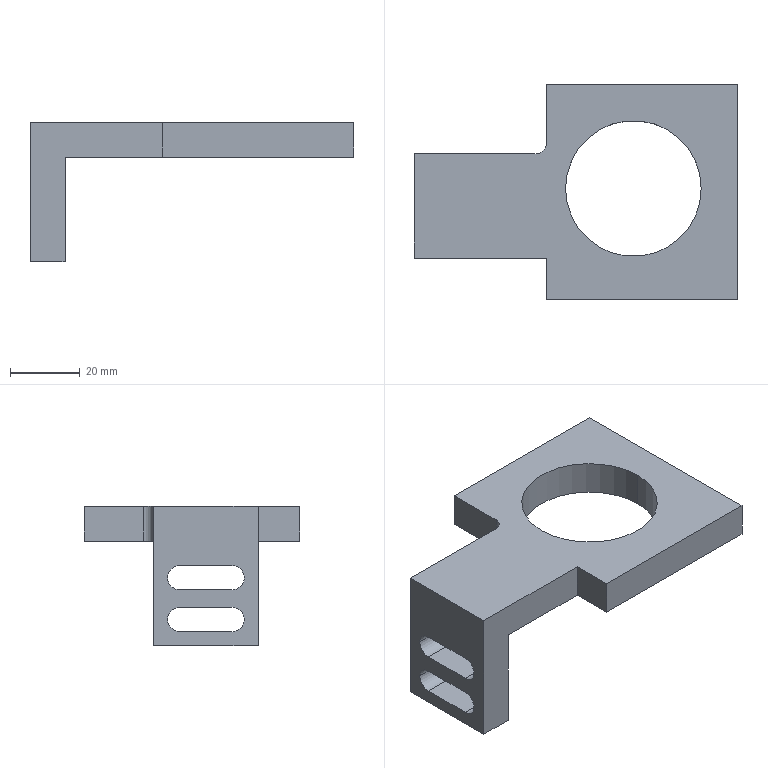Part | SolidWorks | features ICE 5, 3DProfileFeature 1, Extrusion 1, Fillet 1, HoleWzd 1 | 1 solid | 29 faces | box 93 x 62 x 40 mm | volume 39399 mm3 | plane 16 | cylinder 11 | cone 2 | commonest cylinder face diameters 7 x6 5 x2 39 x2 6 x1
STEP:
#1=CARTESIAN_POINT('',(-31.,-35.,-3.5));
#2=VERTEX_POINT('',#1);
#3=CARTESIAN_POINT('',(-31.,-35.,1.5));
#4=VERTEX_POINT('',#3);
#5=CARTESIAN_POINT('',(-31.,-35.,-1.));
#6=DIRECTION('',(0.,1.,0.));
#7=DIRECTION('',(0.,0.,1.));
#8=AXIS2_PLACEMENT_3D('',#5,#6,#7);
#9=CIRCLE('',#8,2.5);
#10=EDGE_CURVE('',#2,#4,#9,.T.);
#11=ORIENTED_EDGE('',*,*,#10,.F.);
#12=CARTESIAN_POINT('',(-31.,-20.,-3.5));
#13=VERTEX_POINT('',#12);
#14=CARTESIAN_POINT('',(-31.,-20.,-3.5));
#15=DIRECTION('',(0.,1.,0.));
#16=VECTOR('',#15,1000.);
#17=LINE('',#14,#16);
#18=EDGE_CURVE('',#2,#13,#17,.T.);
#19=ORIENTED_EDGE('',*,*,#18,.T.);
#20=CARTESIAN_POINT('',(-31.,-20.,1.5));
#21=VERTEX_POINT('',#20);
#22=CARTESIAN_POINT('',(-31.,-20.,-1.));
#23=DIRECTION('',(0.,1.,0.));
#24=DIRECTION('',(0.,0.,1.));
#25=AXIS2_PLACEMENT_3D('',#22,#23,#24);
#26=CIRCLE('',#25,2.5);
#27=EDGE_CURVE('',#13,#21,#26,.T.);
#28=ORIENTED_EDGE('',*,*,#27,.T.);
#29=CARTESIAN_POINT('',(-31.,-20.,1.5));
#30=DIRECTION('',(0.,1.,0.));
#31=VECTOR('',#30,1000.);
#32=LINE('',#29,#31);
#33=EDGE_CURVE('',#4,#21,#32,.T.);
#34=ORIENTED_EDGE('',*,*,#33,.F.);
#35=EDGE_LOOP('',(#11,#19,#28,#34));
#36=FACE_OUTER_BOUND('',#35,.T.);
#37=CARTESIAN_POINT('',(-31.,-20.,-1.));
#38=DIRECTION('',(0.,1.,0.));
#39=DIRECTION('',(0.,0.,1.));
#40=AXIS2_PLACEMENT_3D('',#37,#38,#39);
#41=CYLINDRICAL_SURFACE('',#40,2.5);
#42=ADVANCED_FACE('',(#36),#41,.F.);
#43=CARTESIAN_POINT('',(-31.,-36.502,-1.));
#44=VERTEX_POINT('',#43);
#45=CARTESIAN_POINT('',(-31.,-35.,1.5));
#46=DIRECTION('',(0.,0.515,0.8572));
#47=VECTOR('',#46,1000.);
#48=LINE('',#45,#47);
#49=EDGE_CURVE('',#44,#4,#48,.T.);
#50=ORIENTED_EDGE('',*,*,#49,.F.);
#51=CARTESIAN_POINT('',(-31.,-35.,-3.5));
#52=DIRECTION('',(0.,0.515,-0.8572));
#53=VECTOR('',#52,1000.);
#54=LINE('',#51,#53);
#55=EDGE_CURVE('',#44,#2,#54,.T.);
#56=ORIENTED_EDGE('',*,*,#55,.T.);
#57=ORIENTED_EDGE('',*,*,#10,.T.);
#58=EDGE_LOOP('',(#50,#56,#57));
#59=FACE_OUTER_BOUND('',#58,.T.);
#60=CARTESIAN_POINT('',(-31.,-35.,-1.));
#61=DIRECTION('',(0.,1.,0.));
#62=DIRECTION('',(0.,0.,1.));
#63=AXIS2_PLACEMENT_3D('',#60,#61,#62);
#64=CONICAL_SURFACE('',#63,2.5,1.03);
#65=ADVANCED_FACE('',(#59),#64,.F.);
#66=CARTESIAN_POINT('',(-38.,-27.5,-24.));
#67=VERTEX_POINT('',#66);
#68=CARTESIAN_POINT('',(-38.,-24.,-27.5));
#69=VERTEX_POINT('',#68);
#70=CARTESIAN_POINT('',(-38.,-27.5,-27.5));
#71=DIRECTION('',(-1.,0.,0.));
#72=DIRECTION('',(0.,0.,-1.));
#73=AXIS2_PLACEMENT_3D('',#70,#71,#72);
#74=CIRCLE('',#73,3.5);
#75=EDGE_CURVE('',#67,#69,#74,.T.);
#76=ORIENTED_EDGE('',*,*,#75,.T.);
#77=CARTESIAN_POINT('',(-28.,-24.,-27.5));
#78=VERTEX_POINT('',#77);
#79=CARTESIAN_POINT('',(-38.001,-24.,-27.5));
#80=DIRECTION('',(1.,0.,0.));
#81=VECTOR('',#80,1000.);
#82=LINE('',#79,#81);
#83=EDGE_CURVE('',#69,#78,#82,.T.);
#84=ORIENTED_EDGE('',*,*,#83,.T.);
#85=CARTESIAN_POINT('',(-28.,-27.5,-24.));
#86=VERTEX_POINT('',#85);
#87=CARTESIAN_POINT('',(-28.,-27.5,-27.5));
#88=DIRECTION('',(1.,0.,0.));
#89=DIRECTION('',(0.,1.,0.));
#90=AXIS2_PLACEMENT_3D('',#87,#88,#89);
#91=CIRCLE('',#90,3.5);
#92=EDGE_CURVE('',#78,#86,#91,.T.);
#93=ORIENTED_EDGE('',*,*,#92,.T.);
#94=CARTESIAN_POINT('',(-38.001,-27.5,-24.));
#95=DIRECTION('',(1.,0.,0.));
#96=VECTOR('',#95,1000.);
#97=LINE('',#94,#96);
#98=EDGE_CURVE('',#67,#86,#97,.T.);
#99=ORIENTED_EDGE('',*,*,#98,.F.);
#100=EDGE_LOOP('',(#76,#84,#93,#99));
#101=FACE_OUTER_BOUND('',#100,.T.);
#102=CARTESIAN_POINT('',(-38.001,-27.5,-27.5));
#103=DIRECTION('',(1.,0.,0.));
#104=DIRECTION('',(0.,1.,0.));
#105=AXIS2_PLACEMENT_3D('',#102,#103,#104);
#106=CYLINDRICAL_SURFACE('',#105,3.5);
#107=ADVANCED_FACE('',(#101),#106,.F.);
#108=CARTESIAN_POINT('',(-38.,-27.5,-12.));
#109=VERTEX_POINT('',#108);
#110=CARTESIAN_POINT('',(-38.,-24.,-15.5));
#111=VERTEX_POINT('',#110);
#112=CARTESIAN_POINT('',(-38.,-27.5,-15.5));
#113=DIRECTION('',(-1.,0.,0.));
#114=DIRECTION('',(0.,0.,-1.));
#115=AXIS2_PLACEMENT_3D('',#112,#113,#114);
#116=CIRCLE('',#115,3.5);
#117=EDGE_CURVE('',#109,#111,#116,.T.);
#118=ORIENTED_EDGE('',*,*,#117,.T.);
#119=CARTESIAN_POINT('',(-28.,-24.,-15.5));
#120=VERTEX_POINT('',#119);
#121=CARTESIAN_POINT('',(-38.001,-24.,-15.5));
#122=DIRECTION('',(1.,0.,0.));
#123=VECTOR('',#122,1000.);
#124=LINE('',#121,#123);
#125=EDGE_CURVE('',#111,#120,#124,.T.);
#126=ORIENTED_EDGE('',*,*,#125,.T.);
#127=CARTESIAN_POINT('',(-28.,-27.5,-12.));
#128=VERTEX_POINT('',#127);
#129=CARTESIAN_POINT('',(-28.,-27.5,-15.5));
#130=DIRECTION('',(1.,0.,0.));
#131=DIRECTION('',(0.,1.,0.));
#132=AXIS2_PLACEMENT_3D('',#129,#130,#131);
#133=CIRCLE('',#132,3.5);
#134=EDGE_CURVE('',#120,#128,#133,.T.);
#135=ORIENTED_EDGE('',*,*,#134,.T.);
#136=CARTESIAN_POINT('',(-38.001,-27.5,-12.));
#137=DIRECTION('',(1.,0.,0.));
#138=VECTOR('',#137,1000.);
#139=LINE('',#136,#138);
#140=EDGE_CURVE('',#109,#128,#139,.T.);
#141=ORIENTED_EDGE('',*,*,#140,.F.);
#142=EDGE_LOOP('',(#118,#126,#135,#141));
#143=FACE_OUTER_BOUND('',#142,.T.);
#144=CARTESIAN_POINT('',(-38.001,-27.5,-15.5));
#145=DIRECTION('',(1.,0.,0.));
#146=DIRECTION('',(0.,1.,0.));
#147=AXIS2_PLACEMENT_3D('',#144,#145,#146);
#148=CYLINDRICAL_SURFACE('',#147,3.5);
#149=ADVANCED_FACE('',(#143),#148,.F.);
#150=CARTESIAN_POINT('',(5.5,-30.,5.));
#151=VERTEX_POINT('',#150);
#152=CARTESIAN_POINT('',(44.5,-30.,5.));
#153=VERTEX_POINT('',#152);
#154=CARTESIAN_POINT('',(25.,-30.,5.));
#155=DIRECTION('',(0.,0.,1.));
#156=DIRECTION('',(-1.,0.,0.));
#157=AXIS2_PLACEMENT_3D('',#154,#155,#156);
#158=CIRCLE('',#157,19.5);
#159=EDGE_CURVE('',#151,#153,#158,.T.);
#160=ORIENTED_EDGE('',*,*,#159,.T.);
#161=CARTESIAN_POINT('',(44.5,-30.,-5.));
#162=VERTEX_POINT('',#161);
#163=CARTESIAN_POINT('',(44.5,-30.,5.001));
#164=DIRECTION('',(0.,0.,-1.));
#165=VECTOR('',#164,1000.);
#166=LINE('',#163,#165);
#167=EDGE_CURVE('',#153,#162,#166,.T.);
#168=ORIENTED_EDGE('',*,*,#167,.T.);
#169=CARTESIAN_POINT('',(5.5,-30.,-5.));
#170=VERTEX_POINT('',#169);
#171=CARTESIAN_POINT('',(25.,-30.,-5.));
#172=DIRECTION('',(0.,0.,-1.));
#173=DIRECTION('',(-1.,0.,0.));
#174=AXIS2_PLACEMENT_3D('',#171,#172,#173);
#175=CIRCLE('',#174,19.5);
#176=EDGE_CURVE('',#162,#170,#175,.T.);
#177=ORIENTED_EDGE('',*,*,#176,.T.);
#178=CARTESIAN_POINT('',(5.5,-30.,5.001));
#179=DIRECTION('',(0.,0.,-1.));
#180=VECTOR('',#179,1000.);
#181=LINE('',#178,#180);
#182=EDGE_CURVE('',#151,#170,#181,.T.);
#183=ORIENTED_EDGE('',*,*,#182,.F.);
#184=EDGE_LOOP('',(#160,#168,#177,#183));
#185=FACE_OUTER_BOUND('',#184,.T.);
#186=CARTESIAN_POINT('',(25.,-30.,5.001));
#187=DIRECTION('',(0.,0.,-1.));
#188=DIRECTION('',(-1.,0.,0.));
#189=AXIS2_PLACEMENT_3D('',#186,#187,#188);
#190=CYLINDRICAL_SURFACE('',#189,19.5);
#191=ADVANCED_FACE('',(#185),#190,.F.);
#192=CARTESIAN_POINT('',(0.,-50.,5.));
#193=VERTEX_POINT('',#192);
#194=CARTESIAN_POINT('',(0.,-50.,-5.));
#195=VERTEX_POINT('',#194);
#196=CARTESIAN_POINT('',(0.,-50.,5.));
#197=DIRECTION('',(0.,0.,-1.));
#198=VECTOR('',#197,1000.);
#199=LINE('',#196,#198);
#200=EDGE_CURVE('',#193,#195,#199,.T.);
#201=ORIENTED_EDGE('',*,*,#200,.F.);
#202=CARTESIAN_POINT('',(-38.,-50.,5.));
#203=VERTEX_POINT('',#202);
#204=CARTESIAN_POINT('',(55.,-50.,5.));
#205=DIRECTION('',(1.,0.,0.));
#206=VECTOR('',#205,1000.);
#207=LINE('',#204,#206);
#208=EDGE_CURVE('',#203,#193,#207,.T.);
#209=ORIENTED_EDGE('',*,*,#208,.F.);
#210=CARTESIAN_POINT('',(-38.,-50.,-35.));
#211=VERTEX_POINT('',#210);
#212=CARTESIAN_POINT('',(-38.,-50.,5.));
#213=DIRECTION('',(0.,0.,-1.));
#214=VECTOR('',#213,1000.);
#215=LINE('',#212,#214);
#216=EDGE_CURVE('',#203,#211,#215,.T.);
#217=ORIENTED_EDGE('',*,*,#216,.T.);
#218=CARTESIAN_POINT('',(-28.,-50.,-35.));
#219=VERTEX_POINT('',#218);
#220=CARTESIAN_POINT('',(-38.,-50.,-35.));
#221=DIRECTION('',(-1.,0.,0.));
#222=VECTOR('',#221,1000.);
#223=LINE('',#220,#222);
#224=EDGE_CURVE('',#219,#211,#223,.T.);
#225=ORIENTED_EDGE('',*,*,#224,.F.);
#226=CARTESIAN_POINT('',(-28.,-50.,-5.));
#227=VERTEX_POINT('',#226);
#228=CARTESIAN_POINT('',(-28.,-50.,-35.));
#229=DIRECTION('',(0.,0.,1.));
#230=VECTOR('',#229,1000.);
#231=LINE('',#228,#230);
#232=EDGE_CURVE('',#219,#227,#231,.T.);
#233=ORIENTED_EDGE('',*,*,#232,.T.);
#234=CARTESIAN_POINT('',(55.,-50.,-5.));
#235=DIRECTION('',(1.,0.,0.));
#236=VECTOR('',#235,1000.);
#237=LINE('',#234,#236);
#238=EDGE_CURVE('',#227,#195,#237,.T.);
#239=ORIENTED_EDGE('',*,*,#238,.T.);
#240=EDGE_LOOP('',(#201,#209,#217,#225,#233,#239));
#241=FACE_OUTER_BOUND('',#240,.T.);
#242=CARTESIAN_POINT('',(55.,-50.,5.));
#243=DIRECTION('',(0.,1.,0.));
#244=DIRECTION('',(-1.,0.,0.));
#245=AXIS2_PLACEMENT_3D('',#242,#243,#244);
#246=PLANE('',#245);
#247=ADVANCED_FACE('',(#241),#246,.F.);
#248=CARTESIAN_POINT('',(0.,0.,-5.));
#249=VERTEX_POINT('',#248);
#250=CARTESIAN_POINT('',(0.,-17.,-5.));
#251=VERTEX_POINT('',#250);
#252=CARTESIAN_POINT('',(0.,-20.,-5.));
#253=DIRECTION('',(0.,-1.,0.));
#254=VECTOR('',#253,1000.);
#255=LINE('',#252,#254);
#256=EDGE_CURVE('',#249,#251,#255,.T.);
#257=ORIENTED_EDGE('',*,*,#256,.T.);
#258=CARTESIAN_POINT('',(0.,-17.,5.));
#259=VERTEX_POINT('',#258);
#260=CARTESIAN_POINT('',(0.,-17.,5.));
#261=DIRECTION('',(0.,0.,1.));
#262=VECTOR('',#261,1000.);
#263=LINE('',#260,#262);
#264=EDGE_CURVE('',#251,#259,#263,.T.);
#265=ORIENTED_EDGE('',*,*,#264,.T.);
#266=CARTESIAN_POINT('',(0.,0.,5.));
#267=VERTEX_POINT('',#266);
#268=CARTESIAN_POINT('',(0.,-20.,5.));
#269=DIRECTION('',(0.,-1.,0.));
#270=VECTOR('',#269,1000.);
#271=LINE('',#268,#270);
#272=EDGE_CURVE('',#267,#259,#271,.T.);
#273=ORIENTED_EDGE('',*,*,#272,.F.);
#274=CARTESIAN_POINT('',(0.,0.,5.));
#275=DIRECTION('',(0.,0.,-1.));
#276=VECTOR('',#275,1000.);
#277=LINE('',#274,#276);
#278=EDGE_CURVE('',#267,#249,#277,.T.);
#279=ORIENTED_EDGE('',*,*,#278,.T.);
#280=EDGE_LOOP('',(#257,#265,#273,#279));
#281=FACE_OUTER_BOUND('',#280,.T.);
#282=CARTESIAN_POINT('',(0.,-20.,5.));
#283=DIRECTION('',(1.,0.,0.));
#284=DIRECTION('',(0.,0.,-1.));
#285=AXIS2_PLACEMENT_3D('',#282,#283,#284);
#286=PLANE('',#285);
#287=ADVANCED_FACE('',(#281),#286,.F.);
#288=CARTESIAN_POINT('',(-31.,-20.,-1.));
#289=DIRECTION('',(0.,1.,0.));
#290=DIRECTION('',(0.,0.,1.));
#291=AXIS2_PLACEMENT_3D('',#288,#289,#290);
#292=CIRCLE('',#291,2.5);
#293=EDGE_CURVE('',#21,#13,#292,.T.);
#294=ORIENTED_EDGE('',*,*,#293,.F.);
#295=ORIENTED_EDGE('',*,*,#27,.F.);
#296=EDGE_LOOP('',(#294,#295));
#297=FACE_BOUND('',#296,.T.);
#298=CARTESIAN_POINT('',(-3.,-20.,5.));
#299=VERTEX_POINT('',#298);
#300=CARTESIAN_POINT('',(-38.,-20.,5.));
#301=VERTEX_POINT('',#300);
#302=CARTESIAN_POINT('',(-38.,-20.,5.));
#303=DIRECTION('',(-1.,0.,0.));
#304=VECTOR('',#303,1000.);
#305=LINE('',#302,#304);
#306=EDGE_CURVE('',#299,#301,#305,.T.);
#307=ORIENTED_EDGE('',*,*,#306,.F.);
#308=CARTESIAN_POINT('',(-3.,-20.,-5.));
#309=VERTEX_POINT('',#308);
#310=CARTESIAN_POINT('',(-3.,-20.,-5.));
#311=DIRECTION('',(0.,0.,-1.));
#312=VECTOR('',#311,1000.);
#313=LINE('',#310,#312);
#314=EDGE_CURVE('',#299,#309,#313,.T.);
#315=ORIENTED_EDGE('',*,*,#314,.T.);
#316=CARTESIAN_POINT('',(-28.,-20.,-5.));
#317=VERTEX_POINT('',#316);
#318=CARTESIAN_POINT('',(-38.,-20.,-5.));
#319=DIRECTION('',(-1.,0.,0.));
#320=VECTOR('',#319,1000.);
#321=LINE('',#318,#320);
#322=EDGE_CURVE('',#309,#317,#321,.T.);
#323=ORIENTED_EDGE('',*,*,#322,.T.);
#324=CARTESIAN_POINT('',(-28.,-20.,-35.));
#325=VERTEX_POINT('',#324);
#326=CARTESIAN_POINT('',(-28.,-20.,-35.));
#327=DIRECTION('',(0.,0.,1.));
#328=VECTOR('',#327,1000.);
#329=LINE('',#326,#328);
#330=EDGE_CURVE('',#325,#317,#329,.T.);
#331=ORIENTED_EDGE('',*,*,#330,.F.);
#332=CARTESIAN_POINT('',(-38.,-20.,-35.));
#333=VERTEX_POINT('',#332);
#334=CARTESIAN_POINT('',(-38.,-20.,-35.));
#335=DIRECTION('',(1.,0.,0.));
#336=VECTOR('',#335,1000.);
#337=LINE('',#334,#336);
#338=EDGE_CURVE('',#333,#325,#337,.T.);
#339=ORIENTED_EDGE('',*,*,#338,.F.);
#340=CARTESIAN_POINT('',(-38.,-20.,5.));
#341=DIRECTION('',(0.,0.,-1.));
#342=VECTOR('',#341,1000.);
#343=LINE('',#340,#342);
#344=EDGE_CURVE('',#301,#333,#343,.T.);
#345=ORIENTED_EDGE('',*,*,#344,.F.);
#346=EDGE_LOOP('',(#307,#315,#323,#331,#339,#345));
#347=FACE_OUTER_BOUND('',#346,.T.);
#348=CARTESIAN_POINT('',(-38.,-20.,5.));
#349=DIRECTION('',(0.,-1.,0.));
#350=DIRECTION('',(0.,0.,-1.));
#351=AXIS2_PLACEMENT_3D('',#348,#349,#350);
#352=PLANE('',#351);
#353=ADVANCED_FACE('',(#297,#347),#352,.F.);
#354=CARTESIAN_POINT('',(-38.,-27.5,-31.));
#355=VERTEX_POINT('',#354);
#356=CARTESIAN_POINT('',(-38.,-42.5,-31.));
#357=VERTEX_POINT('',#356);
#358=CARTESIAN_POINT('',(-38.,-27.5,-31.));
#359=DIRECTION('',(0.,-1.,0.));
#360=VECTOR('',#359,1000.);
#361=LINE('',#358,#360);
#362=EDGE_CURVE('',#355,#357,#361,.T.);
#363=ORIENTED_EDGE('',*,*,#362,.F.);
#364=CARTESIAN_POINT('',(-38.,-27.5,-27.5));
#365=DIRECTION('',(-1.,0.,0.));
#366=DIRECTION('',(0.,0.,-1.));
#367=AXIS2_PLACEMENT_3D('',#364,#365,#366);
#368=CIRCLE('',#367,3.5);
#369=EDGE_CURVE('',#69,#355,#368,.T.);
#370=ORIENTED_EDGE('',*,*,#369,.F.);
#371=ORIENTED_EDGE('',*,*,#75,.F.);
#372=CARTESIAN_POINT('',(-38.,-42.5,-24.));
#373=VERTEX_POINT('',#372);
#374=CARTESIAN_POINT('',(-38.,-27.5,-24.));
#375=DIRECTION('',(0.,1.,0.));
#376=VECTOR('',#375,1000.);
#377=LINE('',#374,#376);
#378=EDGE_CURVE('',#373,#67,#377,.T.);
#379=ORIENTED_EDGE('',*,*,#378,.F.);
#380=CARTESIAN_POINT('',(-38.,-42.5,-27.5));
#381=DIRECTION('',(-1.,0.,0.));
#382=DIRECTION('',(0.,0.,-1.));
#383=AXIS2_PLACEMENT_3D('',#380,#381,#382);
#384=CIRCLE('',#383,3.5);
#385=EDGE_CURVE('',#357,#373,#384,.T.);
#386=ORIENTED_EDGE('',*,*,#385,.F.);
#387=EDGE_LOOP('',(#363,#370,#371,#379,#386));
#388=FACE_BOUND('',#387,.T.);
#389=CARTESIAN_POINT('',(-38.,-27.5,-19.));
#390=VERTEX_POINT('',#389);
#391=CARTESIAN_POINT('',(-38.,-42.5,-19.));
#392=VERTEX_POINT('',#391);
#393=CARTESIAN_POINT('',(-38.,-27.5,-19.));
#394=DIRECTION('',(0.,-1.,0.));
#395=VECTOR('',#394,1000.);
#396=LINE('',#393,#395);
#397=EDGE_CURVE('',#390,#392,#396,.T.);
#398=ORIENTED_EDGE('',*,*,#397,.F.);
#399=CARTESIAN_POINT('',(-38.,-27.5,-15.5));
#400=DIRECTION('',(-1.,0.,0.));
#401=DIRECTION('',(0.,0.,-1.));
#402=AXIS2_PLACEMENT_3D('',#399,#400,#401);
#403=CIRCLE('',#402,3.5);
#404=EDGE_CURVE('',#111,#390,#403,.T.);
#405=ORIENTED_EDGE('',*,*,#404,.F.);
#406=ORIENTED_EDGE('',*,*,#117,.F.);
#407=CARTESIAN_POINT('',(-38.,-42.5,-12.));
#408=VERTEX_POINT('',#407);
#409=CARTESIAN_POINT('',(-38.,-27.5,-12.));
#410=DIRECTION('',(0.,1.,0.));
#411=VECTOR('',#410,1000.);
#412=LINE('',#409,#411);
#413=EDGE_CURVE('',#408,#109,#412,.T.);
#414=ORIENTED_EDGE('',*,*,#413,.F.);
#415=CARTESIAN_POINT('',(-38.,-42.5,-15.5));
#416=DIRECTION('',(-1.,0.,0.));
#417=DIRECTION('',(0.,0.,-1.));
#418=AXIS2_PLACEMENT_3D('',#415,#416,#417);
#419=CIRCLE('',#418,3.5);
#420=EDGE_CURVE('',#392,#408,#419,.T.);
#421=ORIENTED_EDGE('',*,*,#420,.F.);
#422=EDGE_LOOP('',(#398,#405,#406,#414,#421));
#423=FACE_BOUND('',#422,.T.);
#424=ORIENTED_EDGE('',*,*,#344,.T.);
#425=CARTESIAN_POINT('',(-38.,-20.,-35.));
#426=DIRECTION('',(0.,1.,0.));
#427=VECTOR('',#426,1000.);
#428=LINE('',#425,#427);
#429=EDGE_CURVE('',#211,#333,#428,.T.);
#430=ORIENTED_EDGE('',*,*,#429,.F.);
#431=ORIENTED_EDGE('',*,*,#216,.F.);
#432=CARTESIAN_POINT('',(-38.,-50.,5.));
#433=DIRECTION('',(0.,-1.,0.));
#434=VECTOR('',#433,1000.);
#435=LINE('',#432,#434);
#436=EDGE_CURVE('',#301,#203,#435,.T.);
#437=ORIENTED_EDGE('',*,*,#436,.F.);
#438=EDGE_LOOP('',(#424,#430,#431,#437));
#439=FACE_OUTER_BOUND('',#438,.T.);
#440=CARTESIAN_POINT('',(-38.,-50.,5.));
#441=DIRECTION('',(1.,0.,0.));
#442=DIRECTION('',(0.,0.,-1.));
#443=AXIS2_PLACEMENT_3D('',#440,#441,#442);
#444=PLANE('',#443);
#445=ADVANCED_FACE('',(#388,#423,#439),#444,.F.);
#446=CARTESIAN_POINT('',(55.,-62.,-5.));
#447=VERTEX_POINT('',#446);
#448=CARTESIAN_POINT('',(55.,0.,-5.));
#449=VERTEX_POINT('',#448);
#450=CARTESIAN_POINT('',(55.,0.,-5.));
#451=DIRECTION('',(0.,1.,0.));
#452=VECTOR('',#451,1000.);
#453=LINE('',#450,#452);
#454=EDGE_CURVE('',#447,#449,#453,.T.);
#455=ORIENTED_EDGE('',*,*,#454,.T.);
#456=CARTESIAN_POINT('',(55.,0.,5.));
#457=VERTEX_POINT('',#456);
#458=CARTESIAN_POINT('',(55.,0.,5.));
#459=DIRECTION('',(0.,0.,-1.));
#460=VECTOR('',#459,1000.);
#461=LINE('',#458,#460);
#462=EDGE_CURVE('',#457,#449,#461,.T.);
#463=ORIENTED_EDGE('',*,*,#462,.F.);
#464=CARTESIAN_POINT('',(55.,-62.,5.));
#465=VERTEX_POINT('',#464);
#466=CARTESIAN_POINT('',(55.,0.,5.));
#467=DIRECTION('',(0.,1.,0.));
#468=VECTOR('',#467,1000.);
#469=LINE('',#466,#468);
#470=EDGE_CURVE('',#465,#457,#469,.T.);
#471=ORIENTED_EDGE('',*,*,#470,.F.);
#472=CARTESIAN_POINT('',(55.,-62.,5.));
#473=DIRECTION('',(0.,0.,1.));
#474=VECTOR('',#473,1000.);
#475=LINE('',#472,#474);
#476=EDGE_CURVE('',#447,#465,#475,.T.);
#477=ORIENTED_EDGE('',*,*,#476,.F.);
#478=EDGE_LOOP('',(#455,#463,#471,#477));
#479=FACE_OUTER_BOUND('',#478,.T.);
#480=CARTESIAN_POINT('',(55.,0.,5.));
#481=DIRECTION('',(-1.,0.,0.));
#482=DIRECTION('',(0.,-1.,0.));
#483=AXIS2_PLACEMENT_3D('',#480,#481,#482);
#484=PLANE('',#483);
#485=ADVANCED_FACE('',(#479),#484,.F.);
#486=CARTESIAN_POINT('',(0.,0.,-5.));
#487=DIRECTION('',(-1.,0.,0.));
#488=VECTOR('',#487,1000.);
#489=LINE('',#486,#488);
#490=EDGE_CURVE('',#449,#249,#489,.T.);
#491=ORIENTED_EDGE('',*,*,#490,.T.);
#492=ORIENTED_EDGE('',*,*,#278,.F.);
#493=CARTESIAN_POINT('',(0.,0.,5.));
#494=DIRECTION('',(-1.,0.,0.));
#495=VECTOR('',#494,1000.);
#496=LINE('',#493,#495);
#497=EDGE_CURVE('',#457,#267,#496,.T.);
#498=ORIENTED_EDGE('',*,*,#497,.F.);
#499=ORIENTED_EDGE('',*,*,#462,.T.);
#500=EDGE_LOOP('',(#491,#492,#498,#499));
#501=FACE_OUTER_BOUND('',#500,.T.);
#502=CARTESIAN_POINT('',(0.,0.,5.));
#503=DIRECTION('',(0.,-1.,0.));
#504=DIRECTION('',(0.,0.,-1.));
#505=AXIS2_PLACEMENT_3D('',#502,#503,#504);
#506=PLANE('',#505);
#507=ADVANCED_FACE('',(#501),#506,.F.);
#508=ORIENTED_EDGE('',*,*,#159,.F.);
#509=CARTESIAN_POINT('',(25.,-30.,5.));
#510=DIRECTION('',(0.,0.,1.));
#511=DIRECTION('',(-1.,0.,0.));
#512=AXIS2_PLACEMENT_3D('',#509,#510,#511);
#513=CIRCLE('',#512,19.5);
#514=EDGE_CURVE('',#153,#151,#513,.T.);
#515=ORIENTED_EDGE('',*,*,#514,.F.);
#516=EDGE_LOOP('',(#508,#515));
#517=FACE_BOUND('',#516,.T.);
#518=ORIENTED_EDGE('',*,*,#272,.T.);
#519=CARTESIAN_POINT('',(-3.,-17.,5.));
#520=DIRECTION('',(0.,0.,-1.));
#521=DIRECTION('',(-1.,0.,0.));
#522=AXIS2_PLACEMENT_3D('',#519,#520,#521);
#523=CIRCLE('',#522,3.);
#524=EDGE_CURVE('',#259,#299,#523,.T.);
#525=ORIENTED_EDGE('',*,*,#524,.T.);
#526=ORIENTED_EDGE('',*,*,#306,.T.);
#527=ORIENTED_EDGE('',*,*,#436,.T.);
#528=ORIENTED_EDGE('',*,*,#208,.T.);
#529=CARTESIAN_POINT('',(0.,-62.,5.));
#530=VERTEX_POINT('',#529);
#531=CARTESIAN_POINT('',(0.,-62.,5.));
#532=DIRECTION('',(0.,1.,0.));
#533=VECTOR('',#532,1000.);
#534=LINE('',#531,#533);
#535=EDGE_CURVE('',#530,#193,#534,.T.);
#536=ORIENTED_EDGE('',*,*,#535,.F.);
#537=CARTESIAN_POINT('',(55.,-62.,5.));
#538=DIRECTION('',(-1.,0.,0.));
#539=VECTOR('',#538,1000.);
#540=LINE('',#537,#539);
#541=EDGE_CURVE('',#465,#530,#540,.T.);
#542=ORIENTED_EDGE('',*,*,#541,.F.);
#543=ORIENTED_EDGE('',*,*,#470,.T.);
#544=ORIENTED_EDGE('',*,*,#497,.T.);
#545=EDGE_LOOP('',(#518,#525,#526,#527,#528,#536,#542,#543,#544));
#546=FACE_OUTER_BOUND('',#545,.T.);
#547=CARTESIAN_POINT('',(0.,0.,5.));
#548=DIRECTION('',(0.,0.,-1.));
#549=DIRECTION('',(-1.,0.,0.));
#550=AXIS2_PLACEMENT_3D('',#547,#548,#549);
#551=PLANE('',#550);
#552=ADVANCED_FACE('',(#517,#546),#551,.F.);
#553=CARTESIAN_POINT('',(-28.,-20.,-5.));
#554=DIRECTION('',(0.,-1.,0.));
#555=VECTOR('',#554,1000.);
#556=LINE('',#553,#555);
#557=EDGE_CURVE('',#317,#227,#556,.T.);
#558=ORIENTED_EDGE('',*,*,#557,.F.);
#559=ORIENTED_EDGE('',*,*,#322,.F.);
#560=CARTESIAN_POINT('',(-3.,-17.,-5.));
#561=DIRECTION('',(0.,0.,1.));
#562=DIRECTION('',(-1.,0.,0.));
#563=AXIS2_PLACEMENT_3D('',#560,#561,#562);
#564=CIRCLE('',#563,3.);
#565=EDGE_CURVE('',#309,#251,#564,.T.);
#566=ORIENTED_EDGE('',*,*,#565,.T.);
#567=ORIENTED_EDGE('',*,*,#256,.F.);
#568=ORIENTED_EDGE('',*,*,#490,.F.);
#569=ORIENTED_EDGE('',*,*,#454,.F.);
#570=CARTESIAN_POINT('',(0.,-62.,-5.));
#571=VERTEX_POINT('',#570);
#572=CARTESIAN_POINT('',(55.,-62.,-5.));
#573=DIRECTION('',(1.,0.,0.));
#574=VECTOR('',#573,1000.);
#575=LINE('',#572,#574);
#576=EDGE_CURVE('',#571,#447,#575,.T.);
#577=ORIENTED_EDGE('',*,*,#576,.F.);
#578=CARTESIAN_POINT('',(0.,-62.,-5.));
#579=DIRECTION('',(0.,1.,0.));
#580=VECTOR('',#579,1000.);
#581=LINE('',#578,#580);
#582=EDGE_CURVE('',#571,#195,#581,.T.);
#583=ORIENTED_EDGE('',*,*,#582,.T.);
#584=ORIENTED_EDGE('',*,*,#238,.F.);
#585=EDGE_LOOP('',(#558,#559,#566,#567,#568,#569,#577,#583,#584));
#586=FACE_OUTER_BOUND('',#585,.T.);
#587=CARTESIAN_POINT('',(25.,-30.,-5.));
#588=DIRECTION('',(0.,0.,-1.));
#589=DIRECTION('',(-1.,0.,0.));
#590=AXIS2_PLACEMENT_3D('',#587,#588,#589);
#591=CIRCLE('',#590,19.5);
#592=EDGE_CURVE('',#170,#162,#591,.T.);
#593=ORIENTED_EDGE('',*,*,#592,.F.);
#594=ORIENTED_EDGE('',*,*,#176,.F.);
#595=EDGE_LOOP('',(#593,#594));
#596=FACE_BOUND('',#595,.T.);
#597=CARTESIAN_POINT('',(0.,0.,-5.));
#598=DIRECTION('',(0.,0.,-1.));
#599=DIRECTION('',(-1.,0.,0.));
#600=AXIS2_PLACEMENT_3D('',#597,#598,#599);
#601=PLANE('',#600);
#602=ADVANCED_FACE('',(#586,#596),#601,.T.);
#603=ORIENTED_EDGE('',*,*,#524,.F.);
#604=ORIENTED_EDGE('',*,*,#264,.F.);
#605=ORIENTED_EDGE('',*,*,#565,.F.);
#606=ORIENTED_EDGE('',*,*,#314,.F.);
#607=EDGE_LOOP('',(#603,#604,#605,#606));
#608=FACE_OUTER_BOUND('',#607,.T.);
#609=CARTESIAN_POINT('',(-3.,-17.,5.));
#610=DIRECTION('',(0.,0.,1.));
#611=DIRECTION('',(1.,0.,0.));
#612=AXIS2_PLACEMENT_3D('',#609,#610,#611);
#613=CYLINDRICAL_SURFACE('',#612,3.);
#614=ADVANCED_FACE('',(#608),#613,.F.);
#615=ORIENTED_EDGE('',*,*,#167,.F.);
#616=ORIENTED_EDGE('',*,*,#514,.T.);
#617=ORIENTED_EDGE('',*,*,#182,.T.);
#618=ORIENTED_EDGE('',*,*,#592,.T.);
#619=EDGE_LOOP('',(#615,#616,#617,#618));
#620=FACE_OUTER_BOUND('',#619,.T.);
#621=CARTESIAN_POINT('',(25.,-30.,5.001));
#622=DIRECTION('',(0.,0.,-1.));
#623=DIRECTION('',(-1.,0.,0.));
#624=AXIS2_PLACEMENT_3D('',#621,#622,#623);
#625=CYLINDRICAL_SURFACE('',#624,19.5);
#626=ADVANCED_FACE('',(#620),#625,.F.);
#627=CARTESIAN_POINT('',(-28.,-42.5,-24.));
#628=VERTEX_POINT('',#627);
#629=CARTESIAN_POINT('',(-28.,-27.5,-24.));
#630=DIRECTION('',(0.,-1.,0.));
#631=VECTOR('',#630,1000.);
#632=LINE('',#629,#631);
#633=EDGE_CURVE('',#86,#628,#632,.T.);
#634=ORIENTED_EDGE('',*,*,#633,.F.);
#635=ORIENTED_EDGE('',*,*,#92,.F.);
#636=CARTESIAN_POINT('',(-28.,-27.5,-31.));
#637=VERTEX_POINT('',#636);
#638=CARTESIAN_POINT('',(-28.,-27.5,-27.5));
#639=DIRECTION('',(1.,0.,0.));
#640=DIRECTION('',(0.,1.,0.));
#641=AXIS2_PLACEMENT_3D('',#638,#639,#640);
#642=CIRCLE('',#641,3.5);
#643=EDGE_CURVE('',#637,#78,#642,.T.);
#644=ORIENTED_EDGE('',*,*,#643,.F.);
#645=CARTESIAN_POINT('',(-28.,-42.5,-31.));
#646=VERTEX_POINT('',#645);
#647=CARTESIAN_POINT('',(-28.,-27.5,-31.));
#648=DIRECTION('',(0.,1.,0.));
#649=VECTOR('',#648,1000.);
#650=LINE('',#647,#649);
#651=EDGE_CURVE('',#646,#637,#650,.T.);
#652=ORIENTED_EDGE('',*,*,#651,.F.);
#653=CARTESIAN_POINT('',(-28.,-42.5,-27.5));
#654=DIRECTION('',(1.,0.,0.));
#655=DIRECTION('',(0.,1.,0.));
#656=AXIS2_PLACEMENT_3D('',#653,#654,#655);
#657=CIRCLE('',#656,3.5);
#658=EDGE_CURVE('',#628,#646,#657,.T.);
#659=ORIENTED_EDGE('',*,*,#658,.F.);
#660=EDGE_LOOP('',(#634,#635,#644,#652,#659));
#661=FACE_BOUND('',#660,.T.);
#662=CARTESIAN_POINT('',(-28.,-42.5,-12.));
#663=VERTEX_POINT('',#662);
#664=CARTESIAN_POINT('',(-28.,-27.5,-12.));
#665=DIRECTION('',(0.,-1.,0.));
#666=VECTOR('',#665,1000.);
#667=LINE('',#664,#666);
#668=EDGE_CURVE('',#128,#663,#667,.T.);
#669=ORIENTED_EDGE('',*,*,#668,.F.);
#670=ORIENTED_EDGE('',*,*,#134,.F.);
#671=CARTESIAN_POINT('',(-28.,-27.5,-19.));
#672=VERTEX_POINT('',#671);
#673=CARTESIAN_POINT('',(-28.,-27.5,-15.5));
#674=DIRECTION('',(1.,0.,0.));
#675=DIRECTION('',(0.,1.,0.));
#676=AXIS2_PLACEMENT_3D('',#673,#674,#675);
#677=CIRCLE('',#676,3.5);
#678=EDGE_CURVE('',#672,#120,#677,.T.);
#679=ORIENTED_EDGE('',*,*,#678,.F.);
#680=CARTESIAN_POINT('',(-28.,-42.5,-19.));
#681=VERTEX_POINT('',#680);
#682=CARTESIAN_POINT('',(-28.,-27.5,-19.));
#683=DIRECTION('',(0.,1.,0.));
#684=VECTOR('',#683,1000.);
#685=LINE('',#682,#684);
#686=EDGE_CURVE('',#681,#672,#685,.T.);
#687=ORIENTED_EDGE('',*,*,#686,.F.);
#688=CARTESIAN_POINT('',(-28.,-42.5,-15.5));
#689=DIRECTION('',(1.,0.,0.));
#690=DIRECTION('',(0.,1.,0.));
#691=AXIS2_PLACEMENT_3D('',#688,#689,#690);
#692=CIRCLE('',#691,3.5);
#693=EDGE_CURVE('',#663,#681,#692,.T.);
#694=ORIENTED_EDGE('',*,*,#693,.F.);
#695=EDGE_LOOP('',(#669,#670,#679,#687,#694));
#696=FACE_BOUND('',#695,.T.);
#697=ORIENTED_EDGE('',*,*,#557,.T.);
#698=ORIENTED_EDGE('',*,*,#232,.F.);
#699=CARTESIAN_POINT('',(-28.,-20.,-35.));
#700=DIRECTION('',(0.,-1.,0.));
#701=VECTOR('',#700,1000.);
#702=LINE('',#699,#701);
#703=EDGE_CURVE('',#325,#219,#702,.T.);
#704=ORIENTED_EDGE('',*,*,#703,.F.);
#705=ORIENTED_EDGE('',*,*,#330,.T.);
#706=EDGE_LOOP('',(#697,#698,#704,#705));
#707=FACE_OUTER_BOUND('',#706,.T.);
#708=CARTESIAN_POINT('',(-28.,-20.,-35.));
#709=DIRECTION('',(-1.,0.,0.));
#710=DIRECTION('',(0.,-1.,0.));
#711=AXIS2_PLACEMENT_3D('',#708,#709,#710);
#712=PLANE('',#711);
#713=ADVANCED_FACE('',(#661,#696,#707),#712,.F.);
#714=ORIENTED_EDGE('',*,*,#429,.T.);
#715=ORIENTED_EDGE('',*,*,#338,.T.);
#716=ORIENTED_EDGE('',*,*,#703,.T.);
#717=ORIENTED_EDGE('',*,*,#224,.T.);
#718=EDGE_LOOP('',(#714,#715,#716,#717));
#719=FACE_OUTER_BOUND('',#718,.T.);
#720=CARTESIAN_POINT('',(0.,0.,-35.));
#721=DIRECTION('',(0.,0.,1.));
#722=DIRECTION('',(1.,0.,0.));
#723=AXIS2_PLACEMENT_3D('',#720,#721,#722);
#724=PLANE('',#723);
#725=ADVANCED_FACE('',(#719),#724,.F.);
#726=ORIENTED_EDGE('',*,*,#125,.F.);
#727=ORIENTED_EDGE('',*,*,#404,.T.);
#728=CARTESIAN_POINT('',(-38.001,-27.5,-19.));
#729=DIRECTION('',(1.,0.,0.));
#730=VECTOR('',#729,1000.);
#731=LINE('',#728,#730);
#732=EDGE_CURVE('',#390,#672,#731,.T.);
#733=ORIENTED_EDGE('',*,*,#732,.T.);
#734=ORIENTED_EDGE('',*,*,#678,.T.);
#735=EDGE_LOOP('',(#726,#727,#733,#734));
#736=FACE_OUTER_BOUND('',#735,.T.);
#737=CARTESIAN_POINT('',(-38.001,-27.5,-15.5));
#738=DIRECTION('',(1.,0.,0.));
#739=DIRECTION('',(0.,1.,0.));
#740=AXIS2_PLACEMENT_3D('',#737,#738,#739);
#741=CYLINDRICAL_SURFACE('',#740,3.5);
#742=ADVANCED_FACE('',(#736),#741,.F.);
#743=ORIENTED_EDGE('',*,*,#397,.T.);
#744=CARTESIAN_POINT('',(-38.001,-42.5,-19.));
#745=DIRECTION('',(1.,0.,0.));
#746=VECTOR('',#745,1000.);
#747=LINE('',#744,#746);
#748=EDGE_CURVE('',#392,#681,#747,.T.);
#749=ORIENTED_EDGE('',*,*,#748,.T.);
#750=ORIENTED_EDGE('',*,*,#686,.T.);
#751=ORIENTED_EDGE('',*,*,#732,.F.);
#752=EDGE_LOOP('',(#743,#749,#750,#751));
#753=FACE_OUTER_BOUND('',#752,.T.);
#754=CARTESIAN_POINT('',(-38.001,-27.5,-19.));
#755=DIRECTION('',(0.,0.,-1.));
#756=DIRECTION('',(-1.,0.,0.));
#757=AXIS2_PLACEMENT_3D('',#754,#755,#756);
#758=PLANE('',#757);
#759=ADVANCED_FACE('',(#753),#758,.F.);
#760=ORIENTED_EDGE('',*,*,#420,.T.);
#761=CARTESIAN_POINT('',(-38.001,-42.5,-12.));
#762=DIRECTION('',(1.,0.,0.));
#763=VECTOR('',#762,1000.);
#764=LINE('',#761,#763);
#765=EDGE_CURVE('',#408,#663,#764,.T.);
#766=ORIENTED_EDGE('',*,*,#765,.T.);
#767=ORIENTED_EDGE('',*,*,#693,.T.);
#768=ORIENTED_EDGE('',*,*,#748,.F.);
#769=EDGE_LOOP('',(#760,#766,#767,#768));
#770=FACE_OUTER_BOUND('',#769,.T.);
#771=CARTESIAN_POINT('',(-38.001,-42.5,-15.5));
#772=DIRECTION('',(1.,0.,0.));
#773=DIRECTION('',(0.,1.,0.));
#774=AXIS2_PLACEMENT_3D('',#771,#772,#773);
#775=CYLINDRICAL_SURFACE('',#774,3.5);
#776=ADVANCED_FACE('',(#770),#775,.F.);
#777=ORIENTED_EDGE('',*,*,#413,.T.);
#778=ORIENTED_EDGE('',*,*,#140,.T.);
#779=ORIENTED_EDGE('',*,*,#668,.T.);
#780=ORIENTED_EDGE('',*,*,#765,.F.);
#781=EDGE_LOOP('',(#777,#778,#779,#780));
#782=FACE_OUTER_BOUND('',#781,.T.);
#783=CARTESIAN_POINT('',(-38.001,-27.5,-12.));
#784=DIRECTION('',(0.,0.,1.));
#785=DIRECTION('',(1.,0.,0.));
#786=AXIS2_PLACEMENT_3D('',#783,#784,#785);
#787=PLANE('',#786);
#788=ADVANCED_FACE('',(#782),#787,.F.);
#789=ORIENTED_EDGE('',*,*,#83,.F.);
#790=ORIENTED_EDGE('',*,*,#369,.T.);
#791=CARTESIAN_POINT('',(-38.001,-27.5,-31.));
#792=DIRECTION('',(1.,0.,0.));
#793=VECTOR('',#792,1000.);
#794=LINE('',#791,#793);
#795=EDGE_CURVE('',#355,#637,#794,.T.);
#796=ORIENTED_EDGE('',*,*,#795,.T.);
#797=ORIENTED_EDGE('',*,*,#643,.T.);
#798=EDGE_LOOP('',(#789,#790,#796,#797));
#799=FACE_OUTER_BOUND('',#798,.T.);
#800=CARTESIAN_POINT('',(-38.001,-27.5,-27.5));
#801=DIRECTION('',(1.,0.,0.));
#802=DIRECTION('',(0.,1.,0.));
#803=AXIS2_PLACEMENT_3D('',#800,#801,#802);
#804=CYLINDRICAL_SURFACE('',#803,3.5);
#805=ADVANCED_FACE('',(#799),#804,.F.);
#806=ORIENTED_EDGE('',*,*,#362,.T.);
#807=CARTESIAN_POINT('',(-38.001,-42.5,-31.));
#808=DIRECTION('',(1.,0.,0.));
#809=VECTOR('',#808,1000.);
#810=LINE('',#807,#809);
#811=EDGE_CURVE('',#357,#646,#810,.T.);
#812=ORIENTED_EDGE('',*,*,#811,.T.);
#813=ORIENTED_EDGE('',*,*,#651,.T.);
#814=ORIENTED_EDGE('',*,*,#795,.F.);
#815=EDGE_LOOP('',(#806,#812,#813,#814));
#816=FACE_OUTER_BOUND('',#815,.T.);
#817=CARTESIAN_POINT('',(-38.001,-27.5,-31.));
#818=DIRECTION('',(0.,0.,-1.));
#819=DIRECTION('',(-1.,0.,0.));
#820=AXIS2_PLACEMENT_3D('',#817,#818,#819);
#821=PLANE('',#820);
#822=ADVANCED_FACE('',(#816),#821,.F.);
#823=ORIENTED_EDGE('',*,*,#385,.T.);
#824=CARTESIAN_POINT('',(-38.001,-42.5,-24.));
#825=DIRECTION('',(1.,0.,0.));
#826=VECTOR('',#825,1000.);
#827=LINE('',#824,#826);
#828=EDGE_CURVE('',#373,#628,#827,.T.);
#829=ORIENTED_EDGE('',*,*,#828,.T.);
#830=ORIENTED_EDGE('',*,*,#658,.T.);
#831=ORIENTED_EDGE('',*,*,#811,.F.);
#832=EDGE_LOOP('',(#823,#829,#830,#831));
#833=FACE_OUTER_BOUND('',#832,.T.);
#834=CARTESIAN_POINT('',(-38.001,-42.5,-27.5));
#835=DIRECTION('',(1.,0.,0.));
#836=DIRECTION('',(0.,1.,0.));
#837=AXIS2_PLACEMENT_3D('',#834,#835,#836);
#838=CYLINDRICAL_SURFACE('',#837,3.5);
#839=ADVANCED_FACE('',(#833),#838,.F.);
#840=ORIENTED_EDGE('',*,*,#378,.T.);
#841=ORIENTED_EDGE('',*,*,#98,.T.);
#842=ORIENTED_EDGE('',*,*,#633,.T.);
#843=ORIENTED_EDGE('',*,*,#828,.F.);
#844=EDGE_LOOP('',(#840,#841,#842,#843));
#845=FACE_OUTER_BOUND('',#844,.T.);
#846=CARTESIAN_POINT('',(-38.001,-27.5,-24.));
#847=DIRECTION('',(0.,0.,1.));
#848=DIRECTION('',(0.,-1.,0.));
#849=AXIS2_PLACEMENT_3D('',#846,#847,#848);
#850=PLANE('',#849);
#851=ADVANCED_FACE('',(#845),#850,.F.);
#852=ORIENTED_EDGE('',*,*,#55,.F.);
#853=ORIENTED_EDGE('',*,*,#49,.T.);
#854=CARTESIAN_POINT('',(-31.,-35.,-1.));
#855=DIRECTION('',(0.,1.,0.));
#856=DIRECTION('',(0.,0.,1.));
#857=AXIS2_PLACEMENT_3D('',#854,#855,#856);
#858=CIRCLE('',#857,2.5);
#859=EDGE_CURVE('',#4,#2,#858,.T.);
#860=ORIENTED_EDGE('',*,*,#859,.T.);
#861=EDGE_LOOP('',(#852,#853,#860));
#862=FACE_OUTER_BOUND('',#861,.T.);
#863=CARTESIAN_POINT('',(-31.,-35.,-1.));
#864=DIRECTION('',(0.,1.,0.));
#865=DIRECTION('',(0.,0.,1.));
#866=AXIS2_PLACEMENT_3D('',#863,#864,#865);
#867=CONICAL_SURFACE('',#866,2.5,1.03);
#868=ADVANCED_FACE('',(#862),#867,.F.);
#869=ORIENTED_EDGE('',*,*,#18,.F.);
#870=ORIENTED_EDGE('',*,*,#859,.F.);
#871=ORIENTED_EDGE('',*,*,#33,.T.);
#872=ORIENTED_EDGE('',*,*,#293,.T.);
#873=EDGE_LOOP('',(#869,#870,#871,#872));
#874=FACE_OUTER_BOUND('',#873,.T.);
#875=CARTESIAN_POINT('',(-31.,-20.,-1.));
#876=DIRECTION('',(0.,1.,0.));
#877=DIRECTION('',(0.,0.,1.));
#878=AXIS2_PLACEMENT_3D('',#875,#876,#877);
#879=CYLINDRICAL_SURFACE('',#878,2.5);
#880=ADVANCED_FACE('',(#874),#879,.F.);
#881=ORIENTED_EDGE('',*,*,#200,.T.);
#882=ORIENTED_EDGE('',*,*,#582,.F.);
#883=CARTESIAN_POINT('',(0.,-62.,5.));
#884=DIRECTION('',(0.,0.,-1.));
#885=VECTOR('',#884,1000.);
#886=LINE('',#883,#885);
#887=EDGE_CURVE('',#530,#571,#886,.T.);
#888=ORIENTED_EDGE('',*,*,#887,.F.);
#889=ORIENTED_EDGE('',*,*,#535,.T.);
#890=EDGE_LOOP('',(#881,#882,#888,#889));
#891=FACE_OUTER_BOUND('',#890,.T.);
#892=CARTESIAN_POINT('',(0.,-62.,5.));
#893=DIRECTION('',(1.,0.,0.));
#894=DIRECTION('',(0.,1.,0.));
#895=AXIS2_PLACEMENT_3D('',#892,#893,#894);
#896=PLANE('',#895);
#897=ADVANCED_FACE('',(#891),#896,.F.);
#898=ORIENTED_EDGE('',*,*,#476,.T.);
#899=ORIENTED_EDGE('',*,*,#541,.T.);
#900=ORIENTED_EDGE('',*,*,#887,.T.);
#901=ORIENTED_EDGE('',*,*,#576,.T.);
#902=EDGE_LOOP('',(#898,#899,#900,#901));
#903=FACE_OUTER_BOUND('',#902,.T.);
#904=CARTESIAN_POINT('',(0.,-62.,0.));
#905=DIRECTION('',(0.,1.,0.));
#906=DIRECTION('',(-1.,0.,0.));
#907=AXIS2_PLACEMENT_3D('',#904,#905,#906);
#908=PLANE('',#907);
#909=ADVANCED_FACE('',(#903),#908,.F.);
#910=CLOSED_SHELL('',(#42,#65,#107,#149,#191,#247,#287,#353,#445,#485,#507,#552,#602,#614,#626,#713,#725,#742,#759,#776,#788,#805,#822,#839,#851,#868,#880,#897,#909));
#911=MANIFOLD_SOLID_BREP('',#910);
#912=CARTESIAN_POINT('',(0.,0.,0.));
#913=DIRECTION('',(0.,0.,1.));
#914=DIRECTION('',(1.,0.,0.));
#915=AXIS2_PLACEMENT_3D('',#912,#913,#914);
#916=(LENGTH_UNIT()NAMED_UNIT(*)SI_UNIT(.MILLI.,.METRE.));
#917=UNCERTAINTY_MEASURE_WITH_UNIT(LENGTH_MEASURE(0.00001),#916,'','');
#918=(NAMED_UNIT(*)PLANE_ANGLE_UNIT()SI_UNIT($,.RADIAN.));
#919=(NAMED_UNIT(*)SI_UNIT($,.STERADIAN.)SOLID_ANGLE_UNIT());
#920=(GEOMETRIC_REPRESENTATION_CONTEXT(3)GLOBAL_UNCERTAINTY_ASSIGNED_CONTEXT((#917))GLOBAL_UNIT_ASSIGNED_CONTEXT((#916,#918,#919))REPRESENTATION_CONTEXT('',''));
#921=ADVANCED_BREP_SHAPE_REPRESENTATION('',(#911,#915),#920);